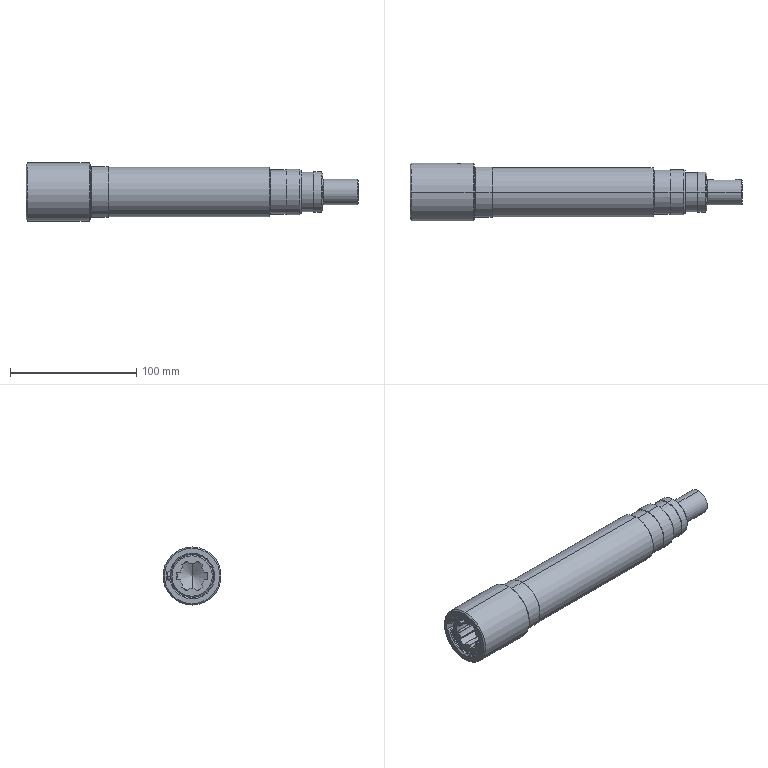Part | SolidWorks | features BaseBody 3 | 3 solids | 176 faces | box 263 x 46 x 46 mm | volume 218227 mm3 | cylinder 90 | plane 47 | cone 39 | commonest cylinder face diameters 0.2 x28 34 x10 20 x9 7 x8 24.739 x6 39 x4